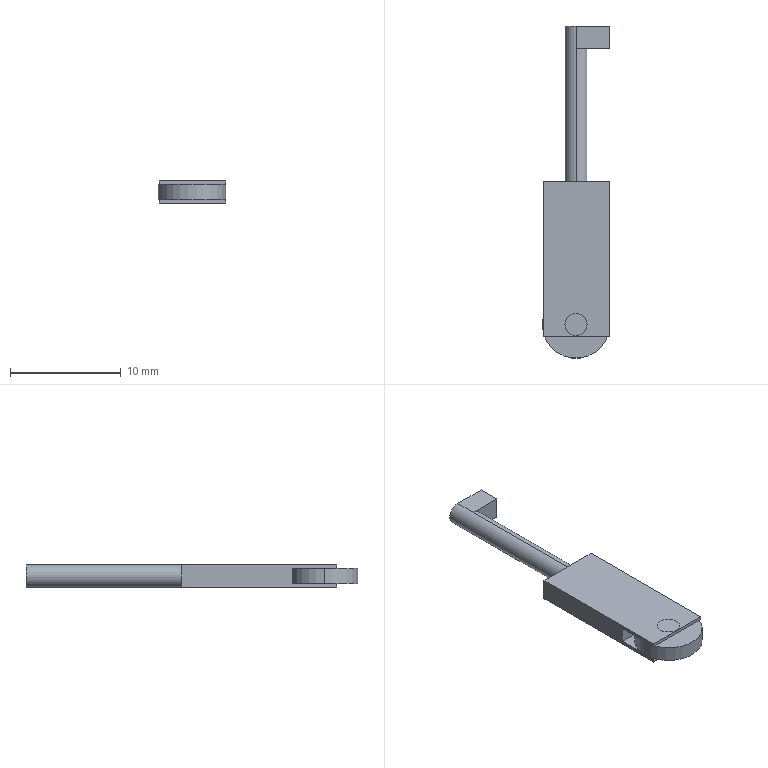Part | SolidWorks | features ICE 3, Cut 2, BaseBody 1 | 3 solids | 32 faces | box 6.079 x 29.943 x 2 mm | volume 227.878 mm3 | plane 20 | cylinder 12 | commonest cylinder face diameters 2 x10 6.079 x2
STEP:
#1=CARTESIAN_POINT('',(-117.509,213.397,177.7));
#2=VERTEX_POINT('',#1);
#3=CARTESIAN_POINT('',(-115.509,213.397,177.7));
#4=VERTEX_POINT('',#3);
#5=CARTESIAN_POINT('',(-116.509,213.397,177.7));
#6=DIRECTION('',(0.,0.,1.));
#7=DIRECTION('',(1.,0.,0.));
#8=AXIS2_PLACEMENT_3D('',#5,#6,#7);
#9=CIRCLE('',#8,1.);
#10=EDGE_CURVE('',#2,#4,#9,.T.);
#11=ORIENTED_EDGE('',*,*,#10,.T.);
#12=CARTESIAN_POINT('',(-115.509,213.397,176.3));
#13=VERTEX_POINT('',#12);
#14=CARTESIAN_POINT('',(-115.509,213.397,177.7));
#15=DIRECTION('',(0.,0.,-1.));
#16=VECTOR('',#15,1000.);
#17=LINE('',#14,#16);
#18=EDGE_CURVE('',#4,#13,#17,.T.);
#19=ORIENTED_EDGE('',*,*,#18,.T.);
#20=CARTESIAN_POINT('',(-117.509,213.397,176.3));
#21=VERTEX_POINT('',#20);
#22=CARTESIAN_POINT('',(-116.509,213.397,176.3));
#23=DIRECTION('',(0.,0.,1.));
#24=DIRECTION('',(1.,0.,0.));
#25=AXIS2_PLACEMENT_3D('',#22,#23,#24);
#26=CIRCLE('',#25,1.);
#27=EDGE_CURVE('',#21,#13,#26,.T.);
#28=ORIENTED_EDGE('',*,*,#27,.F.);
#29=CARTESIAN_POINT('',(-117.509,213.397,177.7));
#30=DIRECTION('',(0.,0.,-1.));
#31=VECTOR('',#30,1000.);
#32=LINE('',#29,#31);
#33=EDGE_CURVE('',#2,#21,#32,.T.);
#34=ORIENTED_EDGE('',*,*,#33,.F.);
#35=EDGE_LOOP('',(#11,#19,#28,#34));
#36=FACE_OUTER_BOUND('',#35,.T.);
#37=CARTESIAN_POINT('',(-116.509,213.397,177.7));
#38=DIRECTION('',(0.,0.,-1.));
#39=DIRECTION('',(-1.,0.,0.));
#40=AXIS2_PLACEMENT_3D('',#37,#38,#39);
#41=CYLINDRICAL_SURFACE('',#40,1.);
#42=ADVANCED_FACE('',(#36),#41,.F.);
#43=CARTESIAN_POINT('',(-113.47,213.397,177.7));
#44=VERTEX_POINT('',#43);
#45=CARTESIAN_POINT('',(-119.549,213.397,177.7));
#46=VERTEX_POINT('',#45);
#47=CARTESIAN_POINT('',(-116.509,213.397,177.7));
#48=DIRECTION('',(0.,0.,1.));
#49=DIRECTION('',(1.,0.,0.));
#50=AXIS2_PLACEMENT_3D('',#47,#48,#49);
#51=CIRCLE('',#50,3.04);
#52=EDGE_CURVE('',#44,#46,#51,.T.);
#53=ORIENTED_EDGE('',*,*,#52,.F.);
#54=CARTESIAN_POINT('',(-113.47,213.397,176.3));
#55=VERTEX_POINT('',#54);
#56=CARTESIAN_POINT('',(-113.47,213.397,177.7));
#57=DIRECTION('',(0.,0.,-1.));
#58=VECTOR('',#57,1000.);
#59=LINE('',#56,#58);
#60=EDGE_CURVE('',#44,#55,#59,.T.);
#61=ORIENTED_EDGE('',*,*,#60,.T.);
#62=CARTESIAN_POINT('',(-119.549,213.397,176.3));
#63=VERTEX_POINT('',#62);
#64=CARTESIAN_POINT('',(-116.509,213.397,176.3));
#65=DIRECTION('',(0.,0.,1.));
#66=DIRECTION('',(1.,0.,0.));
#67=AXIS2_PLACEMENT_3D('',#64,#65,#66);
#68=CIRCLE('',#67,3.04);
#69=EDGE_CURVE('',#55,#63,#68,.T.);
#70=ORIENTED_EDGE('',*,*,#69,.T.);
#71=CARTESIAN_POINT('',(-119.549,213.397,177.7));
#72=DIRECTION('',(0.,0.,-1.));
#73=VECTOR('',#72,1000.);
#74=LINE('',#71,#73);
#75=EDGE_CURVE('',#46,#63,#74,.T.);
#76=ORIENTED_EDGE('',*,*,#75,.F.);
#77=EDGE_LOOP('',(#53,#61,#70,#76));
#78=FACE_OUTER_BOUND('',#77,.T.);
#79=CARTESIAN_POINT('',(-116.509,213.397,177.7));
#80=DIRECTION('',(0.,0.,-1.));
#81=DIRECTION('',(-1.,0.,0.));
#82=AXIS2_PLACEMENT_3D('',#79,#80,#81);
#83=CYLINDRICAL_SURFACE('',#82,3.04);
#84=ADVANCED_FACE('',(#78),#83,.T.);
#85=CARTESIAN_POINT('',(-116.509,213.397,177.7));
#86=DIRECTION('',(0.,0.,1.));
#87=DIRECTION('',(1.,0.,0.));
#88=AXIS2_PLACEMENT_3D('',#85,#86,#87);
#89=CIRCLE('',#88,3.04);
#90=EDGE_CURVE('',#46,#44,#89,.T.);
#91=ORIENTED_EDGE('',*,*,#90,.T.);
#92=ORIENTED_EDGE('',*,*,#52,.T.);
#93=EDGE_LOOP('',(#91,#92));
#94=FACE_OUTER_BOUND('',#93,.T.);
#95=ORIENTED_EDGE('',*,*,#10,.F.);
#96=CARTESIAN_POINT('',(-116.509,213.397,177.7));
#97=DIRECTION('',(0.,0.,1.));
#98=DIRECTION('',(1.,0.,0.));
#99=AXIS2_PLACEMENT_3D('',#96,#97,#98);
#100=CIRCLE('',#99,1.);
#101=EDGE_CURVE('',#4,#2,#100,.T.);
#102=ORIENTED_EDGE('',*,*,#101,.F.);
#103=EDGE_LOOP('',(#95,#102));
#104=FACE_BOUND('',#103,.T.);
#105=CARTESIAN_POINT('',(-116.509,213.397,177.7));
#106=DIRECTION('',(0.,0.,1.));
#107=DIRECTION('',(1.,0.,0.));
#108=AXIS2_PLACEMENT_3D('',#105,#106,#107);
#109=PLANE('',#108);
#110=ADVANCED_FACE('',(#94,#104),#109,.T.);
#111=CARTESIAN_POINT('',(-116.509,213.397,176.3));
#112=DIRECTION('',(0.,0.,1.));
#113=DIRECTION('',(1.,0.,0.));
#114=AXIS2_PLACEMENT_3D('',#111,#112,#113);
#115=CIRCLE('',#114,3.04);
#116=EDGE_CURVE('',#63,#55,#115,.T.);
#117=ORIENTED_EDGE('',*,*,#116,.F.);
#118=ORIENTED_EDGE('',*,*,#69,.F.);
#119=EDGE_LOOP('',(#117,#118));
#120=FACE_OUTER_BOUND('',#119,.T.);
#121=ORIENTED_EDGE('',*,*,#27,.T.);
#122=CARTESIAN_POINT('',(-116.509,213.397,176.3));
#123=DIRECTION('',(0.,0.,1.));
#124=DIRECTION('',(1.,0.,0.));
#125=AXIS2_PLACEMENT_3D('',#122,#123,#124);
#126=CIRCLE('',#125,1.);
#127=EDGE_CURVE('',#13,#21,#126,.T.);
#128=ORIENTED_EDGE('',*,*,#127,.T.);
#129=EDGE_LOOP('',(#121,#128));
#130=FACE_BOUND('',#129,.T.);
#131=CARTESIAN_POINT('',(-116.509,213.397,176.3));
#132=DIRECTION('',(0.,0.,1.));
#133=DIRECTION('',(1.,0.,0.));
#134=AXIS2_PLACEMENT_3D('',#131,#132,#133);
#135=PLANE('',#134);
#136=ADVANCED_FACE('',(#120,#130),#135,.F.);
#137=ORIENTED_EDGE('',*,*,#60,.F.);
#138=ORIENTED_EDGE('',*,*,#90,.F.);
#139=ORIENTED_EDGE('',*,*,#75,.T.);
#140=ORIENTED_EDGE('',*,*,#116,.T.);
#141=EDGE_LOOP('',(#137,#138,#139,#140));
#142=FACE_OUTER_BOUND('',#141,.T.);
#143=CARTESIAN_POINT('',(-116.509,213.397,177.7));
#144=DIRECTION('',(0.,0.,-1.));
#145=DIRECTION('',(-1.,0.,0.));
#146=AXIS2_PLACEMENT_3D('',#143,#144,#145);
#147=CYLINDRICAL_SURFACE('',#146,3.04);
#148=ADVANCED_FACE('',(#142),#147,.T.);
#149=ORIENTED_EDGE('',*,*,#18,.F.);
#150=ORIENTED_EDGE('',*,*,#101,.T.);
#151=ORIENTED_EDGE('',*,*,#33,.T.);
#152=ORIENTED_EDGE('',*,*,#127,.F.);
#153=EDGE_LOOP('',(#149,#150,#151,#152));
#154=FACE_OUTER_BOUND('',#153,.T.);
#155=CARTESIAN_POINT('',(-116.509,213.397,177.7));
#156=DIRECTION('',(0.,0.,-1.));
#157=DIRECTION('',(-1.,0.,0.));
#158=AXIS2_PLACEMENT_3D('',#155,#156,#157);
#159=CYLINDRICAL_SURFACE('',#158,1.);
#160=ADVANCED_FACE('',(#154),#159,.F.);
#161=CLOSED_SHELL('',(#42,#84,#110,#136,#148,#160));
#162=MANIFOLD_SOLID_BREP('',#161);
#163=CARTESIAN_POINT('',(-117.509,213.397,177.7));
#164=VERTEX_POINT('',#163);
#165=CARTESIAN_POINT('',(-115.509,213.397,177.7));
#166=VERTEX_POINT('',#165);
#167=CARTESIAN_POINT('',(-116.509,213.397,177.7));
#168=DIRECTION('',(0.,0.,1.));
#169=DIRECTION('',(1.,0.,0.));
#170=AXIS2_PLACEMENT_3D('',#167,#168,#169);
#171=CIRCLE('',#170,1.);
#172=EDGE_CURVE('',#164,#166,#171,.T.);
#173=ORIENTED_EDGE('',*,*,#172,.F.);
#174=CARTESIAN_POINT('',(-117.509,213.397,178.));
#175=VERTEX_POINT('',#174);
#176=CARTESIAN_POINT('',(-117.509,213.397,174.6));
#177=DIRECTION('',(0.,0.,1.));
#178=VECTOR('',#177,1000.);
#179=LINE('',#176,#178);
#180=EDGE_CURVE('',#164,#175,#179,.T.);
#181=ORIENTED_EDGE('',*,*,#180,.T.);
#182=CARTESIAN_POINT('',(-115.509,213.397,178.));
#183=VERTEX_POINT('',#182);
#184=CARTESIAN_POINT('',(-116.509,213.397,178.));
#185=DIRECTION('',(0.,0.,1.));
#186=DIRECTION('',(1.,0.,0.));
#187=AXIS2_PLACEMENT_3D('',#184,#185,#186);
#188=CIRCLE('',#187,1.);
#189=EDGE_CURVE('',#175,#183,#188,.T.);
#190=ORIENTED_EDGE('',*,*,#189,.T.);
#191=CARTESIAN_POINT('',(-115.509,213.397,174.6));
#192=DIRECTION('',(0.,0.,1.));
#193=VECTOR('',#192,1000.);
#194=LINE('',#191,#193);
#195=EDGE_CURVE('',#166,#183,#194,.T.);
#196=ORIENTED_EDGE('',*,*,#195,.F.);
#197=EDGE_LOOP('',(#173,#181,#190,#196));
#198=FACE_OUTER_BOUND('',#197,.T.);
#199=CARTESIAN_POINT('',(-116.509,213.397,174.6));
#200=DIRECTION('',(0.,0.,1.));
#201=DIRECTION('',(1.,0.,0.));
#202=AXIS2_PLACEMENT_3D('',#199,#200,#201);
#203=CYLINDRICAL_SURFACE('',#202,1.);
#204=ADVANCED_FACE('',(#198),#203,.F.);
#205=CARTESIAN_POINT('',(-117.509,213.397,176.));
#206=VERTEX_POINT('',#205);
#207=CARTESIAN_POINT('',(-115.509,213.397,176.));
#208=VERTEX_POINT('',#207);
#209=CARTESIAN_POINT('',(-116.509,213.397,176.));
#210=DIRECTION('',(0.,0.,1.));
#211=DIRECTION('',(1.,0.,0.));
#212=AXIS2_PLACEMENT_3D('',#209,#210,#211);
#213=CIRCLE('',#212,1.);
#214=EDGE_CURVE('',#206,#208,#213,.T.);
#215=ORIENTED_EDGE('',*,*,#214,.F.);
#216=CARTESIAN_POINT('',(-117.509,213.397,176.3));
#217=VERTEX_POINT('',#216);
#218=CARTESIAN_POINT('',(-117.509,213.397,174.6));
#219=DIRECTION('',(0.,0.,1.));
#220=VECTOR('',#219,1000.);
#221=LINE('',#218,#220);
#222=EDGE_CURVE('',#206,#217,#221,.T.);
#223=ORIENTED_EDGE('',*,*,#222,.T.);
#224=CARTESIAN_POINT('',(-115.509,213.397,176.3));
#225=VERTEX_POINT('',#224);
#226=CARTESIAN_POINT('',(-116.509,213.397,176.3));
#227=DIRECTION('',(0.,0.,-1.));
#228=DIRECTION('',(-1.,0.,0.));
#229=AXIS2_PLACEMENT_3D('',#226,#227,#228);
#230=CIRCLE('',#229,1.);
#231=EDGE_CURVE('',#225,#217,#230,.T.);
#232=ORIENTED_EDGE('',*,*,#231,.F.);
#233=CARTESIAN_POINT('',(-115.509,213.397,174.6));
#234=DIRECTION('',(0.,0.,1.));
#235=VECTOR('',#234,1000.);
#236=LINE('',#233,#235);
#237=EDGE_CURVE('',#208,#225,#236,.T.);
#238=ORIENTED_EDGE('',*,*,#237,.F.);
#239=EDGE_LOOP('',(#215,#223,#232,#238));
#240=FACE_OUTER_BOUND('',#239,.T.);
#241=CARTESIAN_POINT('',(-116.509,213.397,174.6));
#242=DIRECTION('',(0.,0.,1.));
#243=DIRECTION('',(1.,0.,0.));
#244=AXIS2_PLACEMENT_3D('',#241,#242,#243);
#245=CYLINDRICAL_SURFACE('',#244,1.);
#246=ADVANCED_FACE('',(#240),#245,.F.);
#247=CARTESIAN_POINT('',(-116.47,226.3,176.));
#248=VERTEX_POINT('',#247);
#249=CARTESIAN_POINT('',(-116.47,226.3,178.));
#250=VERTEX_POINT('',#249);
#251=CARTESIAN_POINT('',(-116.47,226.3,177.));
#252=DIRECTION('',(0.,-1.,0.));
#253=DIRECTION('',(0.,0.,1.));
#254=AXIS2_PLACEMENT_3D('',#251,#252,#253);
#255=CIRCLE('',#254,1.);
#256=EDGE_CURVE('',#248,#250,#255,.T.);
#257=ORIENTED_EDGE('',*,*,#256,.F.);
#258=CARTESIAN_POINT('',(-116.47,238.3,176.));
#259=VERTEX_POINT('',#258);
#260=CARTESIAN_POINT('',(-116.47,224.3,176.));
#261=DIRECTION('',(0.,1.,0.));
#262=VECTOR('',#261,1000.);
#263=LINE('',#260,#262);
#264=EDGE_CURVE('',#248,#259,#263,.T.);
#265=ORIENTED_EDGE('',*,*,#264,.T.);
#266=CARTESIAN_POINT('',(-116.47,238.3,178.));
#267=VERTEX_POINT('',#266);
#268=CARTESIAN_POINT('',(-116.47,238.3,177.));
#269=DIRECTION('',(0.,1.,0.));
#270=DIRECTION('',(0.,0.,1.));
#271=AXIS2_PLACEMENT_3D('',#268,#269,#270);
#272=CIRCLE('',#271,1.);
#273=EDGE_CURVE('',#267,#259,#272,.T.);
#274=ORIENTED_EDGE('',*,*,#273,.F.);
#275=CARTESIAN_POINT('',(-116.47,224.3,178.));
#276=DIRECTION('',(0.,1.,0.));
#277=VECTOR('',#276,1000.);
#278=LINE('',#275,#277);
#279=EDGE_CURVE('',#250,#267,#278,.T.);
#280=ORIENTED_EDGE('',*,*,#279,.F.);
#281=EDGE_LOOP('',(#257,#265,#274,#280));
#282=FACE_OUTER_BOUND('',#281,.T.);
#283=CARTESIAN_POINT('',(-116.47,224.3,177.));
#284=DIRECTION('',(0.,1.,0.));
#285=DIRECTION('',(0.,0.,1.));
#286=AXIS2_PLACEMENT_3D('',#283,#284,#285);
#287=CYLINDRICAL_SURFACE('',#286,1.);
#288=ADVANCED_FACE('',(#282),#287,.T.);
#289=CARTESIAN_POINT('',(-113.47,212.3,177.7));
#290=VERTEX_POINT('',#289);
#291=CARTESIAN_POINT('',(-119.47,212.3,177.7));
#292=VERTEX_POINT('',#291);
#293=CARTESIAN_POINT('',(-119.47,212.3,177.7));
#294=DIRECTION('',(-1.,0.,0.));
#295=VECTOR('',#294,1000.);
#296=LINE('',#293,#295);
#297=EDGE_CURVE('',#290,#292,#296,.T.);
#298=ORIENTED_EDGE('',*,*,#297,.F.);
#299=CARTESIAN_POINT('',(-113.47,212.3,178.));
#300=VERTEX_POINT('',#299);
#301=CARTESIAN_POINT('',(-113.47,212.3,176.));
#302=DIRECTION('',(0.,0.,1.));
#303=VECTOR('',#302,1000.);
#304=LINE('',#301,#303);
#305=EDGE_CURVE('',#290,#300,#304,.T.);
#306=ORIENTED_EDGE('',*,*,#305,.T.);
#307=CARTESIAN_POINT('',(-119.47,212.3,178.));
#308=VERTEX_POINT('',#307);
#309=CARTESIAN_POINT('',(-119.47,212.3,178.));
#310=DIRECTION('',(1.,0.,0.));
#311=VECTOR('',#310,1000.);
#312=LINE('',#309,#311);
#313=EDGE_CURVE('',#308,#300,#312,.T.);
#314=ORIENTED_EDGE('',*,*,#313,.F.);
#315=CARTESIAN_POINT('',(-119.47,212.3,176.));
#316=DIRECTION('',(0.,0.,1.));
#317=VECTOR('',#316,1000.);
#318=LINE('',#315,#317);
#319=EDGE_CURVE('',#292,#308,#318,.T.);
#320=ORIENTED_EDGE('',*,*,#319,.F.);
#321=EDGE_LOOP('',(#298,#306,#314,#320));
#322=FACE_OUTER_BOUND('',#321,.T.);
#323=CARTESIAN_POINT('',(-119.47,212.3,176.));
#324=DIRECTION('',(0.,-1.,0.));
#325=DIRECTION('',(0.,0.,-1.));
#326=AXIS2_PLACEMENT_3D('',#323,#324,#325);
#327=PLANE('',#326);
#328=ADVANCED_FACE('',(#322),#327,.T.);
#329=CARTESIAN_POINT('',(-116.47,240.3,178.));
#330=VERTEX_POINT('',#329);
#331=CARTESIAN_POINT('',(-113.47,240.3,178.));
#332=VERTEX_POINT('',#331);
#333=CARTESIAN_POINT('',(-116.47,240.3,178.));
#334=DIRECTION('',(1.,0.,0.));
#335=VECTOR('',#334,1000.);
#336=LINE('',#333,#335);
#337=EDGE_CURVE('',#330,#332,#336,.T.);
#338=ORIENTED_EDGE('',*,*,#337,.F.);
#339=CARTESIAN_POINT('',(-116.47,238.3,178.));
#340=DIRECTION('',(0.,1.,0.));
#341=VECTOR('',#340,1000.);
#342=LINE('',#339,#341);
#343=EDGE_CURVE('',#267,#330,#342,.T.);
#344=ORIENTED_EDGE('',*,*,#343,.F.);
#345=CARTESIAN_POINT('',(-113.47,238.3,178.));
#346=VERTEX_POINT('',#345);
#347=CARTESIAN_POINT('',(-116.47,238.3,178.));
#348=DIRECTION('',(1.,0.,0.));
#349=VECTOR('',#348,1000.);
#350=LINE('',#347,#349);
#351=EDGE_CURVE('',#267,#346,#350,.T.);
#352=ORIENTED_EDGE('',*,*,#351,.T.);
#353=CARTESIAN_POINT('',(-113.47,238.3,178.));
#354=DIRECTION('',(0.,1.,0.));
#355=VECTOR('',#354,1000.);
#356=LINE('',#353,#355);
#357=EDGE_CURVE('',#346,#332,#356,.T.);
#358=ORIENTED_EDGE('',*,*,#357,.T.);
#359=EDGE_LOOP('',(#338,#344,#352,#358));
#360=FACE_OUTER_BOUND('',#359,.T.);
#361=CARTESIAN_POINT('',(-116.47,238.3,178.));
#362=DIRECTION('',(0.,0.,1.));
#363=DIRECTION('',(1.,0.,0.));
#364=AXIS2_PLACEMENT_3D('',#361,#362,#363);
#365=PLANE('',#364);
#366=ADVANCED_FACE('',(#360),#365,.T.);
#367=CARTESIAN_POINT('',(-113.47,240.3,176.));
#368=VERTEX_POINT('',#367);
#369=CARTESIAN_POINT('',(-113.47,240.3,178.));
#370=DIRECTION('',(0.,0.,-1.));
#371=VECTOR('',#370,1000.);
#372=LINE('',#369,#371);
#373=EDGE_CURVE('',#332,#368,#372,.T.);
#374=ORIENTED_EDGE('',*,*,#373,.F.);
#375=ORIENTED_EDGE('',*,*,#357,.F.);
#376=CARTESIAN_POINT('',(-113.47,238.3,176.));
#377=VERTEX_POINT('',#376);
#378=CARTESIAN_POINT('',(-113.47,238.3,178.));
#379=DIRECTION('',(0.,0.,-1.));
#380=VECTOR('',#379,1000.);
#381=LINE('',#378,#380);
#382=EDGE_CURVE('',#346,#377,#381,.T.);
#383=ORIENTED_EDGE('',*,*,#382,.T.);
#384=CARTESIAN_POINT('',(-113.47,238.3,176.));
#385=DIRECTION('',(0.,1.,0.));
#386=VECTOR('',#385,1000.);
#387=LINE('',#384,#386);
#388=EDGE_CURVE('',#377,#368,#387,.T.);
#389=ORIENTED_EDGE('',*,*,#388,.T.);
#390=EDGE_LOOP('',(#374,#375,#383,#389));
#391=FACE_OUTER_BOUND('',#390,.T.);
#392=CARTESIAN_POINT('',(-113.47,238.3,178.));
#393=DIRECTION('',(1.,0.,0.));
#394=DIRECTION('',(0.,0.,-1.));
#395=AXIS2_PLACEMENT_3D('',#392,#393,#394);
#396=PLANE('',#395);
#397=ADVANCED_FACE('',(#391),#396,.T.);
#398=CARTESIAN_POINT('',(-116.47,240.3,176.));
#399=VERTEX_POINT('',#398);
#400=CARTESIAN_POINT('',(-113.47,240.3,176.));
#401=DIRECTION('',(-1.,0.,0.));
#402=VECTOR('',#401,1000.);
#403=LINE('',#400,#402);
#404=EDGE_CURVE('',#368,#399,#403,.T.);
#405=ORIENTED_EDGE('',*,*,#404,.F.);
#406=ORIENTED_EDGE('',*,*,#388,.F.);
#407=CARTESIAN_POINT('',(-113.47,238.3,176.));
#408=DIRECTION('',(-1.,0.,0.));
#409=VECTOR('',#408,1000.);
#410=LINE('',#407,#409);
#411=EDGE_CURVE('',#377,#259,#410,.T.);
#412=ORIENTED_EDGE('',*,*,#411,.T.);
#413=CARTESIAN_POINT('',(-116.47,238.3,176.));
#414=DIRECTION('',(0.,1.,0.));
#415=VECTOR('',#414,1000.);
#416=LINE('',#413,#415);
#417=EDGE_CURVE('',#259,#399,#416,.T.);
#418=ORIENTED_EDGE('',*,*,#417,.T.);
#419=EDGE_LOOP('',(#405,#406,#412,#418));
#420=FACE_OUTER_BOUND('',#419,.T.);
#421=CARTESIAN_POINT('',(-113.47,238.3,176.));
#422=DIRECTION('',(0.,0.,-1.));
#423=DIRECTION('',(-1.,0.,0.));
#424=AXIS2_PLACEMENT_3D('',#421,#422,#423);
#425=PLANE('',#424);
#426=ADVANCED_FACE('',(#420),#425,.T.);
#427=ORIENTED_EDGE('',*,*,#351,.F.);
#428=ORIENTED_EDGE('',*,*,#273,.T.);
#429=ORIENTED_EDGE('',*,*,#411,.F.);
#430=ORIENTED_EDGE('',*,*,#382,.F.);
#431=EDGE_LOOP('',(#427,#428,#429,#430));
#432=FACE_OUTER_BOUND('',#431,.T.);
#433=CARTESIAN_POINT('',(5.,238.3,27.866));
#434=DIRECTION('',(0.,1.,0.));
#435=DIRECTION('',(0.,0.,1.));
#436=AXIS2_PLACEMENT_3D('',#433,#434,#435);
#437=PLANE('',#436);
#438=ADVANCED_FACE('',(#432),#437,.F.);
#439=ORIENTED_EDGE('',*,*,#404,.T.);
#440=CARTESIAN_POINT('',(-116.47,240.3,177.));
#441=DIRECTION('',(0.,1.,0.));
#442=DIRECTION('',(1.,0.,0.));
#443=AXIS2_PLACEMENT_3D('',#440,#441,#442);
#444=CIRCLE('',#443,1.);
#445=EDGE_CURVE('',#399,#330,#444,.T.);
#446=ORIENTED_EDGE('',*,*,#445,.T.);
#447=ORIENTED_EDGE('',*,*,#337,.T.);
#448=ORIENTED_EDGE('',*,*,#373,.T.);
#449=EDGE_LOOP('',(#439,#446,#447,#448));
#450=FACE_OUTER_BOUND('',#449,.T.);
#451=CARTESIAN_POINT('',(5.,240.3,27.866));
#452=DIRECTION('',(0.,1.,0.));
#453=DIRECTION('',(0.,0.,1.));
#454=AXIS2_PLACEMENT_3D('',#451,#452,#453);
#455=PLANE('',#454);
#456=ADVANCED_FACE('',(#450),#455,.T.);
#457=ORIENTED_EDGE('',*,*,#264,.F.);
#458=CARTESIAN_POINT('',(-116.47,226.3,177.));
#459=DIRECTION('',(0.,-1.,0.));
#460=DIRECTION('',(0.,0.,1.));
#461=AXIS2_PLACEMENT_3D('',#458,#459,#460);
#462=CIRCLE('',#461,1.);
#463=EDGE_CURVE('',#250,#248,#462,.T.);
#464=ORIENTED_EDGE('',*,*,#463,.F.);
#465=ORIENTED_EDGE('',*,*,#279,.T.);
#466=ORIENTED_EDGE('',*,*,#343,.T.);
#467=ORIENTED_EDGE('',*,*,#445,.F.);
#468=ORIENTED_EDGE('',*,*,#417,.F.);
#469=EDGE_LOOP('',(#457,#464,#465,#466,#467,#468));
#470=FACE_OUTER_BOUND('',#469,.T.);
#471=CARTESIAN_POINT('',(-116.47,224.3,177.));
#472=DIRECTION('',(0.,1.,0.));
#473=DIRECTION('',(0.,0.,1.));
#474=AXIS2_PLACEMENT_3D('',#471,#472,#473);
#475=CYLINDRICAL_SURFACE('',#474,1.);
#476=ADVANCED_FACE('',(#470),#475,.T.);
#477=CARTESIAN_POINT('',(-119.47,226.3,178.));
#478=VERTEX_POINT('',#477);
#479=CARTESIAN_POINT('',(-113.47,226.3,178.));
#480=DIRECTION('',(-1.,0.,0.));
#481=VECTOR('',#480,1000.);
#482=LINE('',#479,#481);
#483=EDGE_CURVE('',#250,#478,#482,.T.);
#484=ORIENTED_EDGE('',*,*,#483,.F.);
#485=ORIENTED_EDGE('',*,*,#463,.T.);
#486=CARTESIAN_POINT('',(-119.47,226.3,176.));
#487=VERTEX_POINT('',#486);
#488=CARTESIAN_POINT('',(-113.47,226.3,176.));
#489=DIRECTION('',(-1.,0.,0.));
#490=VECTOR('',#489,1000.);
#491=LINE('',#488,#490);
#492=EDGE_CURVE('',#248,#487,#491,.T.);
#493=ORIENTED_EDGE('',*,*,#492,.T.);
#494=CARTESIAN_POINT('',(-119.47,226.3,176.));
#495=DIRECTION('',(0.,0.,1.));
#496=VECTOR('',#495,1000.);
#497=LINE('',#494,#496);
#498=EDGE_CURVE('',#487,#478,#497,.T.);
#499=ORIENTED_EDGE('',*,*,#498,.T.);
#500=EDGE_LOOP('',(#484,#485,#493,#499));
#501=FACE_OUTER_BOUND('',#500,.T.);
#502=CARTESIAN_POINT('',(-113.47,226.3,176.));
#503=DIRECTION('',(0.,1.,0.));
#504=DIRECTION('',(0.,0.,1.));
#505=AXIS2_PLACEMENT_3D('',#502,#503,#504);
#506=PLANE('',#505);
#507=ADVANCED_FACE('',(#501),#506,.T.);
#508=CARTESIAN_POINT('',(-119.47,216.3,177.7));
#509=VERTEX_POINT('',#508);
#510=CARTESIAN_POINT('',(-119.47,226.3,177.7));
#511=DIRECTION('',(0.,1.,0.));
#512=VECTOR('',#511,1000.);
#513=LINE('',#510,#512);
#514=EDGE_CURVE('',#292,#509,#513,.T.);
#515=ORIENTED_EDGE('',*,*,#514,.F.);
#516=ORIENTED_EDGE('',*,*,#319,.T.);
#517=CARTESIAN_POINT('',(-119.47,226.3,178.));
#518=DIRECTION('',(0.,-1.,0.));
#519=VECTOR('',#518,1000.);
#520=LINE('',#517,#519);
#521=EDGE_CURVE('',#478,#308,#520,.T.);
#522=ORIENTED_EDGE('',*,*,#521,.F.);
#523=ORIENTED_EDGE('',*,*,#498,.F.);
#524=CARTESIAN_POINT('',(-119.47,212.3,176.));
#525=VERTEX_POINT('',#524);
#526=CARTESIAN_POINT('',(-119.47,226.3,176.));
#527=DIRECTION('',(0.,-1.,0.));
#528=VECTOR('',#527,1000.);
#529=LINE('',#526,#528);
#530=EDGE_CURVE('',#487,#525,#529,.T.);
#531=ORIENTED_EDGE('',*,*,#530,.T.);
#532=CARTESIAN_POINT('',(-119.47,212.3,176.3));
#533=VERTEX_POINT('',#532);
#534=CARTESIAN_POINT('',(-119.47,212.3,176.));
#535=DIRECTION('',(0.,0.,1.));
#536=VECTOR('',#535,1000.);
#537=LINE('',#534,#536);
#538=EDGE_CURVE('',#525,#533,#537,.T.);
#539=ORIENTED_EDGE('',*,*,#538,.T.);
#540=CARTESIAN_POINT('',(-119.47,216.3,176.3));
#541=VERTEX_POINT('',#540);
#542=CARTESIAN_POINT('',(-119.47,226.3,176.3));
#543=DIRECTION('',(0.,-1.,0.));
#544=VECTOR('',#543,1000.);
#545=LINE('',#542,#544);
#546=EDGE_CURVE('',#541,#533,#545,.T.);
#547=ORIENTED_EDGE('',*,*,#546,.F.);
#548=CARTESIAN_POINT('',(-119.47,216.3,176.));
#549=DIRECTION('',(0.,0.,1.));
#550=VECTOR('',#549,1000.);
#551=LINE('',#548,#550);
#552=EDGE_CURVE('',#541,#509,#551,.T.);
#553=ORIENTED_EDGE('',*,*,#552,.T.);
#554=EDGE_LOOP('',(#515,#516,#522,#523,#531,#539,#547,#553));
#555=FACE_OUTER_BOUND('',#554,.T.);
#556=CARTESIAN_POINT('',(-119.47,226.3,176.));
#557=DIRECTION('',(-1.,0.,0.));
#558=DIRECTION('',(0.,0.,1.));
#559=AXIS2_PLACEMENT_3D('',#556,#557,#558);
#560=PLANE('',#559);
#561=ADVANCED_FACE('',(#555),#560,.T.);
#562=CARTESIAN_POINT('',(-113.47,216.3,177.7));
#563=VERTEX_POINT('',#562);
#564=CARTESIAN_POINT('',(-113.47,212.3,177.7));
#565=DIRECTION('',(0.,-1.,0.));
#566=VECTOR('',#565,1000.);
#567=LINE('',#564,#566);
#568=EDGE_CURVE('',#563,#290,#567,.T.);
#569=ORIENTED_EDGE('',*,*,#568,.F.);
#570=CARTESIAN_POINT('',(-113.47,216.3,176.3));
#571=VERTEX_POINT('',#570);
#572=CARTESIAN_POINT('',(-113.47,216.3,176.));
#573=DIRECTION('',(0.,0.,-1.));
#574=VECTOR('',#573,1000.);
#575=LINE('',#572,#574);
#576=EDGE_CURVE('',#563,#571,#575,.T.);
#577=ORIENTED_EDGE('',*,*,#576,.T.);
#578=CARTESIAN_POINT('',(-113.47,212.3,176.3));
#579=VERTEX_POINT('',#578);
#580=CARTESIAN_POINT('',(-113.47,212.3,176.3));
#581=DIRECTION('',(0.,1.,0.));
#582=VECTOR('',#581,1000.);
#583=LINE('',#580,#582);
#584=EDGE_CURVE('',#579,#571,#583,.T.);
#585=ORIENTED_EDGE('',*,*,#584,.F.);
#586=CARTESIAN_POINT('',(-113.47,212.3,176.));
#587=VERTEX_POINT('',#586);
#588=CARTESIAN_POINT('',(-113.47,212.3,176.));
#589=DIRECTION('',(0.,0.,1.));
#590=VECTOR('',#589,1000.);
#591=LINE('',#588,#590);
#592=EDGE_CURVE('',#587,#579,#591,.T.);
#593=ORIENTED_EDGE('',*,*,#592,.F.);
#594=CARTESIAN_POINT('',(-113.47,226.3,176.));
#595=VERTEX_POINT('',#594);
#596=CARTESIAN_POINT('',(-113.47,212.3,176.));
#597=DIRECTION('',(0.,1.,0.));
#598=VECTOR('',#597,1000.);
#599=LINE('',#596,#598);
#600=EDGE_CURVE('',#587,#595,#599,.T.);
#601=ORIENTED_EDGE('',*,*,#600,.T.);
#602=CARTESIAN_POINT('',(-113.47,226.3,178.));
#603=VERTEX_POINT('',#602);
#604=CARTESIAN_POINT('',(-113.47,226.3,176.));
#605=DIRECTION('',(0.,0.,1.));
#606=VECTOR('',#605,1000.);
#607=LINE('',#604,#606);
#608=EDGE_CURVE('',#595,#603,#607,.T.);
#609=ORIENTED_EDGE('',*,*,#608,.T.);
#610=CARTESIAN_POINT('',(-113.47,212.3,178.));
#611=DIRECTION('',(0.,1.,0.));
#612=VECTOR('',#611,1000.);
#613=LINE('',#610,#612);
#614=EDGE_CURVE('',#300,#603,#613,.T.);
#615=ORIENTED_EDGE('',*,*,#614,.F.);
#616=ORIENTED_EDGE('',*,*,#305,.F.);
#617=EDGE_LOOP('',(#569,#577,#585,#593,#601,#609,#615,#616));
#618=FACE_OUTER_BOUND('',#617,.T.);
#619=CARTESIAN_POINT('',(-113.47,212.3,176.));
#620=DIRECTION('',(1.,0.,0.));
#621=DIRECTION('',(0.,0.,-1.));
#622=AXIS2_PLACEMENT_3D('',#619,#620,#621);
#623=PLANE('',#622);
#624=ADVANCED_FACE('',(#618),#623,.T.);
#625=CARTESIAN_POINT('',(-113.47,226.3,176.));
#626=DIRECTION('',(-1.,0.,0.));
#627=VECTOR('',#626,1000.);
#628=LINE('',#625,#627);
#629=EDGE_CURVE('',#595,#248,#628,.T.);
#630=ORIENTED_EDGE('',*,*,#629,.T.);
#631=ORIENTED_EDGE('',*,*,#256,.T.);
#632=CARTESIAN_POINT('',(-113.47,226.3,178.));
#633=DIRECTION('',(-1.,0.,0.));
#634=VECTOR('',#633,1000.);
#635=LINE('',#632,#634);
#636=EDGE_CURVE('',#603,#250,#635,.T.);
#637=ORIENTED_EDGE('',*,*,#636,.F.);
#638=ORIENTED_EDGE('',*,*,#608,.F.);
#639=EDGE_LOOP('',(#630,#631,#637,#638));
#640=FACE_OUTER_BOUND('',#639,.T.);
#641=CARTESIAN_POINT('',(-113.47,226.3,176.));
#642=DIRECTION('',(0.,1.,0.));
#643=DIRECTION('',(0.,0.,1.));
#644=AXIS2_PLACEMENT_3D('',#641,#642,#643);
#645=PLANE('',#644);
#646=ADVANCED_FACE('',(#640),#645,.T.);
#647=CARTESIAN_POINT('',(-116.509,213.397,176.));
#648=DIRECTION('',(0.,0.,1.));
#649=DIRECTION('',(1.,0.,0.));
#650=AXIS2_PLACEMENT_3D('',#647,#648,#649);
#651=CIRCLE('',#650,1.);
#652=EDGE_CURVE('',#208,#206,#651,.T.);
#653=ORIENTED_EDGE('',*,*,#652,.T.);
#654=ORIENTED_EDGE('',*,*,#214,.T.);
#655=EDGE_LOOP('',(#653,#654));
#656=FACE_BOUND('',#655,.T.);
#657=ORIENTED_EDGE('',*,*,#600,.F.);
#658=CARTESIAN_POINT('',(-119.47,212.3,176.));
#659=DIRECTION('',(1.,0.,0.));
#660=VECTOR('',#659,1000.);
#661=LINE('',#658,#660);
#662=EDGE_CURVE('',#525,#587,#661,.T.);
#663=ORIENTED_EDGE('',*,*,#662,.F.);
#664=ORIENTED_EDGE('',*,*,#530,.F.);
#665=ORIENTED_EDGE('',*,*,#492,.F.);
#666=ORIENTED_EDGE('',*,*,#629,.F.);
#667=EDGE_LOOP('',(#657,#663,#664,#665,#666));
#668=FACE_OUTER_BOUND('',#667,.T.);
#669=CARTESIAN_POINT('',(5.,0.3,176.));
#670=DIRECTION('',(0.,0.,1.));
#671=DIRECTION('',(1.,0.,0.));
#672=AXIS2_PLACEMENT_3D('',#669,#670,#671);
#673=PLANE('',#672);
#674=ADVANCED_FACE('',(#656,#668),#673,.F.);
#675=CARTESIAN_POINT('',(-116.509,213.397,178.));
#676=DIRECTION('',(0.,0.,1.));
#677=DIRECTION('',(1.,0.,0.));
#678=AXIS2_PLACEMENT_3D('',#675,#676,#677);
#679=CIRCLE('',#678,1.);
#680=EDGE_CURVE('',#183,#175,#679,.T.);
#681=ORIENTED_EDGE('',*,*,#680,.F.);
#682=ORIENTED_EDGE('',*,*,#189,.F.);
#683=EDGE_LOOP('',(#681,#682));
#684=FACE_BOUND('',#683,.T.);
#685=ORIENTED_EDGE('',*,*,#521,.T.);
#686=ORIENTED_EDGE('',*,*,#313,.T.);
#687=ORIENTED_EDGE('',*,*,#614,.T.);
#688=ORIENTED_EDGE('',*,*,#636,.T.);
#689=ORIENTED_EDGE('',*,*,#483,.T.);
#690=EDGE_LOOP('',(#685,#686,#687,#688,#689));
#691=FACE_OUTER_BOUND('',#690,.T.);
#692=CARTESIAN_POINT('',(5.,0.3,178.));
#693=DIRECTION('',(0.,0.,1.));
#694=DIRECTION('',(1.,0.,0.));
#695=AXIS2_PLACEMENT_3D('',#692,#693,#694);
#696=PLANE('',#695);
#697=ADVANCED_FACE('',(#684,#691),#696,.T.);
#698=CARTESIAN_POINT('',(-119.47,212.3,176.3));
#699=DIRECTION('',(1.,0.,0.));
#700=VECTOR('',#699,1000.);
#701=LINE('',#698,#700);
#702=EDGE_CURVE('',#533,#579,#701,.T.);
#703=ORIENTED_EDGE('',*,*,#702,.F.);
#704=ORIENTED_EDGE('',*,*,#538,.F.);
#705=ORIENTED_EDGE('',*,*,#662,.T.);
#706=ORIENTED_EDGE('',*,*,#592,.T.);
#707=EDGE_LOOP('',(#703,#704,#705,#706));
#708=FACE_OUTER_BOUND('',#707,.T.);
#709=CARTESIAN_POINT('',(-119.47,212.3,176.));
#710=DIRECTION('',(0.,-1.,0.));
#711=DIRECTION('',(0.,0.,-1.));
#712=AXIS2_PLACEMENT_3D('',#709,#710,#711);
#713=PLANE('',#712);
#714=ADVANCED_FACE('',(#708),#713,.T.);
#715=CARTESIAN_POINT('',(-116.509,213.397,177.7));
#716=DIRECTION('',(0.,0.,1.));
#717=DIRECTION('',(1.,0.,0.));
#718=AXIS2_PLACEMENT_3D('',#715,#716,#717);
#719=CIRCLE('',#718,1.);
#720=EDGE_CURVE('',#166,#164,#719,.T.);
#721=ORIENTED_EDGE('',*,*,#720,.T.);
#722=ORIENTED_EDGE('',*,*,#172,.T.);
#723=EDGE_LOOP('',(#721,#722));
#724=FACE_BOUND('',#723,.T.);
#725=ORIENTED_EDGE('',*,*,#514,.T.);
#726=CARTESIAN_POINT('',(-120.153,216.3,177.7));
#727=DIRECTION('',(-1.,0.,0.));
#728=VECTOR('',#727,1000.);
#729=LINE('',#726,#728);
#730=EDGE_CURVE('',#563,#509,#729,.T.);
#731=ORIENTED_EDGE('',*,*,#730,.F.);
#732=ORIENTED_EDGE('',*,*,#568,.T.);
#733=ORIENTED_EDGE('',*,*,#297,.T.);
#734=EDGE_LOOP('',(#725,#731,#732,#733));
#735=FACE_OUTER_BOUND('',#734,.T.);
#736=CARTESIAN_POINT('',(-120.153,216.3,177.7));
#737=DIRECTION('',(0.,0.,1.));
#738=DIRECTION('',(1.,0.,0.));
#739=AXIS2_PLACEMENT_3D('',#736,#737,#738);
#740=PLANE('',#739);
#741=ADVANCED_FACE('',(#724,#735),#740,.F.);
#742=ORIENTED_EDGE('',*,*,#231,.T.);
#743=CARTESIAN_POINT('',(-116.509,213.397,176.3));
#744=DIRECTION('',(0.,0.,-1.));
#745=DIRECTION('',(-1.,0.,0.));
#746=AXIS2_PLACEMENT_3D('',#743,#744,#745);
#747=CIRCLE('',#746,1.);
#748=EDGE_CURVE('',#217,#225,#747,.T.);
#749=ORIENTED_EDGE('',*,*,#748,.T.);
#750=EDGE_LOOP('',(#742,#749));
#751=FACE_BOUND('',#750,.T.);
#752=ORIENTED_EDGE('',*,*,#546,.T.);
#753=ORIENTED_EDGE('',*,*,#702,.T.);
#754=ORIENTED_EDGE('',*,*,#584,.T.);
#755=CARTESIAN_POINT('',(-120.153,216.3,176.3));
#756=DIRECTION('',(1.,0.,0.));
#757=VECTOR('',#756,1000.);
#758=LINE('',#755,#757);
#759=EDGE_CURVE('',#541,#571,#758,.T.);
#760=ORIENTED_EDGE('',*,*,#759,.F.);
#761=EDGE_LOOP('',(#752,#753,#754,#760));
#762=FACE_OUTER_BOUND('',#761,.T.);
#763=CARTESIAN_POINT('',(-120.153,216.3,176.3));
#764=DIRECTION('',(0.,0.,-1.));
#765=DIRECTION('',(-1.,0.,0.));
#766=AXIS2_PLACEMENT_3D('',#763,#764,#765);
#767=PLANE('',#766);
#768=ADVANCED_FACE('',(#751,#762),#767,.F.);
#769=ORIENTED_EDGE('',*,*,#759,.T.);
#770=ORIENTED_EDGE('',*,*,#576,.F.);
#771=ORIENTED_EDGE('',*,*,#730,.T.);
#772=ORIENTED_EDGE('',*,*,#552,.F.);
#773=EDGE_LOOP('',(#769,#770,#771,#772));
#774=FACE_OUTER_BOUND('',#773,.T.);
#775=CARTESIAN_POINT('',(0.,216.3,0.));
#776=DIRECTION('',(0.,-1.,0.));
#777=DIRECTION('',(0.,0.,-1.));
#778=AXIS2_PLACEMENT_3D('',#775,#776,#777);
#779=PLANE('',#778);
#780=ADVANCED_FACE('',(#774),#779,.T.);
#781=ORIENTED_EDGE('',*,*,#222,.F.);
#782=ORIENTED_EDGE('',*,*,#652,.F.);
#783=ORIENTED_EDGE('',*,*,#237,.T.);
#784=ORIENTED_EDGE('',*,*,#748,.F.);
#785=EDGE_LOOP('',(#781,#782,#783,#784));
#786=FACE_OUTER_BOUND('',#785,.T.);
#787=CARTESIAN_POINT('',(-116.509,213.397,174.6));
#788=DIRECTION('',(0.,0.,1.));
#789=DIRECTION('',(1.,0.,0.));
#790=AXIS2_PLACEMENT_3D('',#787,#788,#789);
#791=CYLINDRICAL_SURFACE('',#790,1.);
#792=ADVANCED_FACE('',(#786),#791,.F.);
#793=ORIENTED_EDGE('',*,*,#180,.F.);
#794=ORIENTED_EDGE('',*,*,#720,.F.);
#795=ORIENTED_EDGE('',*,*,#195,.T.);
#796=ORIENTED_EDGE('',*,*,#680,.T.);
#797=EDGE_LOOP('',(#793,#794,#795,#796));
#798=FACE_OUTER_BOUND('',#797,.T.);
#799=CARTESIAN_POINT('',(-116.509,213.397,174.6));
#800=DIRECTION('',(0.,0.,1.));
#801=DIRECTION('',(1.,0.,0.));
#802=AXIS2_PLACEMENT_3D('',#799,#800,#801);
#803=CYLINDRICAL_SURFACE('',#802,1.);
#804=ADVANCED_FACE('',(#798),#803,.F.);
#805=CLOSED_SHELL('',(#204,#246,#288,#328,#366,#397,#426,#438,#456,#476,#507,#561,#624,#646,#674,#697,#714,#741,#768,#780,#792,#804));
#806=MANIFOLD_SOLID_BREP('',#805);
#807=CARTESIAN_POINT('',(-115.509,213.397,176.));
#808=VERTEX_POINT('',#807);
#809=CARTESIAN_POINT('',(-117.509,213.397,176.));
#810=VERTEX_POINT('',#809);
#811=CARTESIAN_POINT('',(-116.509,213.397,176.));
#812=DIRECTION('',(0.,0.,1.));
#813=DIRECTION('',(1.,0.,0.));
#814=AXIS2_PLACEMENT_3D('',#811,#812,#813);
#815=CIRCLE('',#814,1.);
#816=EDGE_CURVE('',#808,#810,#815,.T.);
#817=ORIENTED_EDGE('',*,*,#816,.T.);
#818=CARTESIAN_POINT('',(-117.509,213.397,178.));
#819=VERTEX_POINT('',#818);
#820=CARTESIAN_POINT('',(-117.509,213.397,176.));
#821=DIRECTION('',(0.,0.,1.));
#822=VECTOR('',#821,1000.);
#823=LINE('',#820,#822);
#824=EDGE_CURVE('',#810,#819,#823,.T.);
#825=ORIENTED_EDGE('',*,*,#824,.T.);
#826=CARTESIAN_POINT('',(-115.509,213.397,178.));
#827=VERTEX_POINT('',#826);
#828=CARTESIAN_POINT('',(-116.509,213.397,178.));
#829=DIRECTION('',(0.,0.,1.));
#830=DIRECTION('',(1.,0.,0.));
#831=AXIS2_PLACEMENT_3D('',#828,#829,#830);
#832=CIRCLE('',#831,1.);
#833=EDGE_CURVE('',#827,#819,#832,.T.);
#834=ORIENTED_EDGE('',*,*,#833,.F.);
#835=CARTESIAN_POINT('',(-115.509,213.397,176.));
#836=DIRECTION('',(0.,0.,1.));
#837=VECTOR('',#836,1000.);
#838=LINE('',#835,#837);
#839=EDGE_CURVE('',#808,#827,#838,.T.);
#840=ORIENTED_EDGE('',*,*,#839,.F.);
#841=EDGE_LOOP('',(#817,#825,#834,#840));
#842=FACE_OUTER_BOUND('',#841,.T.);
#843=CARTESIAN_POINT('',(-116.509,213.397,176.));
#844=DIRECTION('',(0.,0.,1.));
#845=DIRECTION('',(1.,0.,0.));
#846=AXIS2_PLACEMENT_3D('',#843,#844,#845);
#847=CYLINDRICAL_SURFACE('',#846,1.);
#848=ADVANCED_FACE('',(#842),#847,.T.);
#849=ORIENTED_EDGE('',*,*,#824,.F.);
#850=CARTESIAN_POINT('',(-116.509,213.397,176.));
#851=DIRECTION('',(0.,0.,1.));
#852=DIRECTION('',(1.,0.,0.));
#853=AXIS2_PLACEMENT_3D('',#850,#851,#852);
#854=CIRCLE('',#853,1.);
#855=EDGE_CURVE('',#810,#808,#854,.T.);
#856=ORIENTED_EDGE('',*,*,#855,.T.);
#857=ORIENTED_EDGE('',*,*,#839,.T.);
#858=CARTESIAN_POINT('',(-116.509,213.397,178.));
#859=DIRECTION('',(0.,0.,1.));
#860=DIRECTION('',(1.,0.,0.));
#861=AXIS2_PLACEMENT_3D('',#858,#859,#860);
#862=CIRCLE('',#861,1.);
#863=EDGE_CURVE('',#819,#827,#862,.T.);
#864=ORIENTED_EDGE('',*,*,#863,.F.);
#865=EDGE_LOOP('',(#849,#856,#857,#864));
#866=FACE_OUTER_BOUND('',#865,.T.);
#867=CARTESIAN_POINT('',(-116.509,213.397,176.));
#868=DIRECTION('',(0.,0.,1.));
#869=DIRECTION('',(1.,0.,0.));
#870=AXIS2_PLACEMENT_3D('',#867,#868,#869);
#871=CYLINDRICAL_SURFACE('',#870,1.);
#872=ADVANCED_FACE('',(#866),#871,.T.);
#873=ORIENTED_EDGE('',*,*,#816,.F.);
#874=ORIENTED_EDGE('',*,*,#855,.F.);
#875=EDGE_LOOP('',(#873,#874));
#876=FACE_OUTER_BOUND('',#875,.T.);
#877=CARTESIAN_POINT('',(-116.509,213.397,176.));
#878=DIRECTION('',(0.,0.,1.));
#879=DIRECTION('',(1.,0.,0.));
#880=AXIS2_PLACEMENT_3D('',#877,#878,#879);
#881=PLANE('',#880);
#882=ADVANCED_FACE('',(#876),#881,.F.);
#883=ORIENTED_EDGE('',*,*,#833,.T.);
#884=ORIENTED_EDGE('',*,*,#863,.T.);
#885=EDGE_LOOP('',(#883,#884));
#886=FACE_OUTER_BOUND('',#885,.T.);
#887=CARTESIAN_POINT('',(-116.509,213.397,178.));
#888=DIRECTION('',(0.,0.,1.));
#889=DIRECTION('',(1.,0.,0.));
#890=AXIS2_PLACEMENT_3D('',#887,#888,#889);
#891=PLANE('',#890);
#892=ADVANCED_FACE('',(#886),#891,.T.);
#893=CLOSED_SHELL('',(#848,#872,#882,#892));
#894=MANIFOLD_SOLID_BREP('',#893);
#895=CARTESIAN_POINT('',(0.,0.,0.));
#896=DIRECTION('',(0.,0.,1.));
#897=DIRECTION('',(1.,0.,0.));
#898=AXIS2_PLACEMENT_3D('',#895,#896,#897);
#899=(LENGTH_UNIT()NAMED_UNIT(*)SI_UNIT(.MILLI.,.METRE.));
#900=UNCERTAINTY_MEASURE_WITH_UNIT(LENGTH_MEASURE(0.00001),#899,'','');
#901=(NAMED_UNIT(*)PLANE_ANGLE_UNIT()SI_UNIT($,.RADIAN.));
#902=(NAMED_UNIT(*)SI_UNIT($,.STERADIAN.)SOLID_ANGLE_UNIT());
#903=(GEOMETRIC_REPRESENTATION_CONTEXT(3)GLOBAL_UNCERTAINTY_ASSIGNED_CONTEXT((#900))GLOBAL_UNIT_ASSIGNED_CONTEXT((#899,#901,#902))REPRESENTATION_CONTEXT('',''));
#904=ADVANCED_BREP_SHAPE_REPRESENTATION('',(#162,#806,#894,#898),#903);